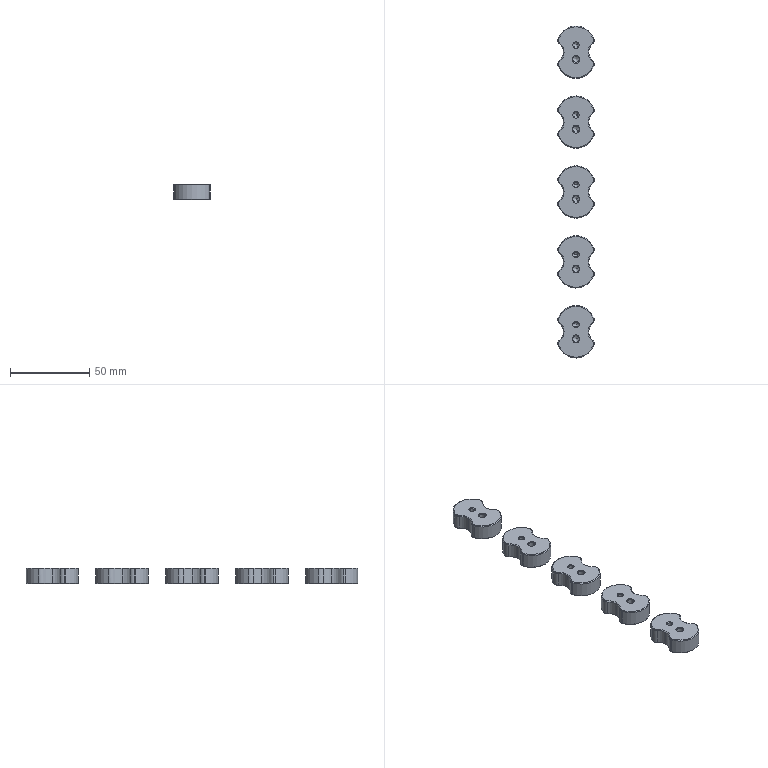NC program | NX | posted with a generic post | part box 22.923 x 209 x 10 mm
Lines 1 to 18 of 9354:
N10 G17 G21 G94 G90
(FLOOR_WALL , TOOL : D80)
N12 T19 M6
N14 G54
N16 G17 G0 G90 X-149.5 Y0. S6500 M3
N18 G43 Z30. H19
N20 Z3.
N22 G94 G1 Z0. F1500.
N24 X-146.5
N26 X146.5
N28 X149.5
N30 Z3.
N32 G0 Z30.
N34 M5